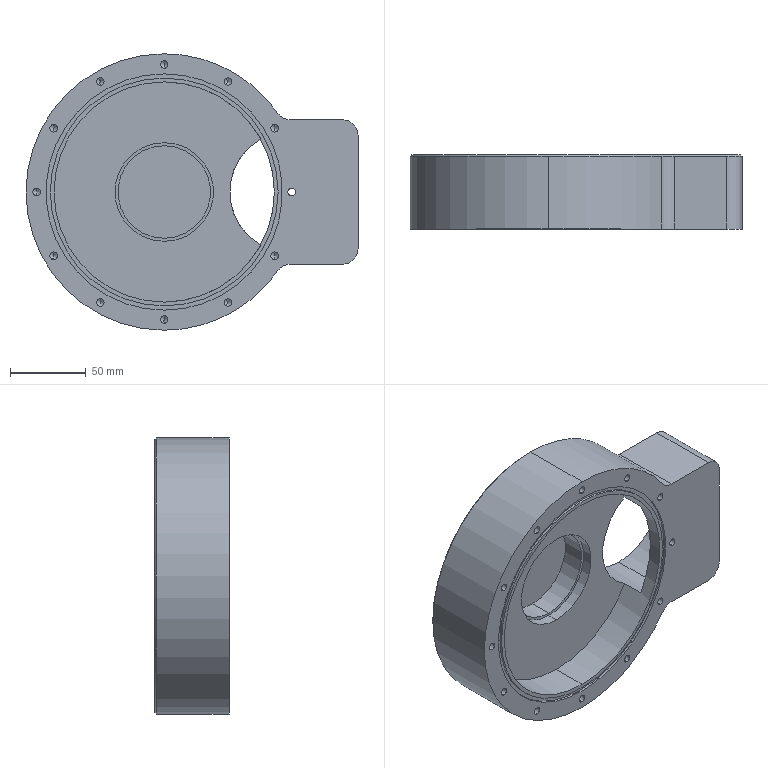Part | SolidWorks | features ICE 4, HoleWzd 2, Chamfer 1, Fillet 1, MoveFace 1, Revolution 1 | 1 solid | 102 faces | box 218.619 x 49 x 182 mm | volume 811897 mm3 | cylinder 51 | cone 37 | plane 14 | commonest cylinder face diameters 5 x24 6.8 x8 20 x4 182 x3 61 x2 65 x2